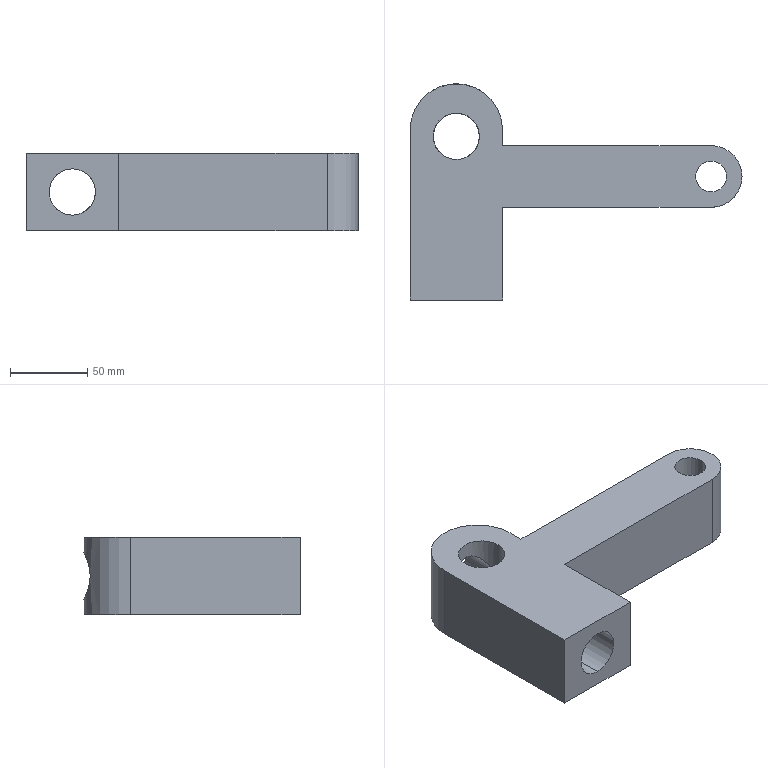Part | STEP file | Imported16 | 1 solid | 21 faces | box 215 x 140 x 50 mm | volume 570776 mm3 | cylinder 13 | plane 8 | commonest cylinder face diameters 30 x8 20 x2 40 x2 60 x1